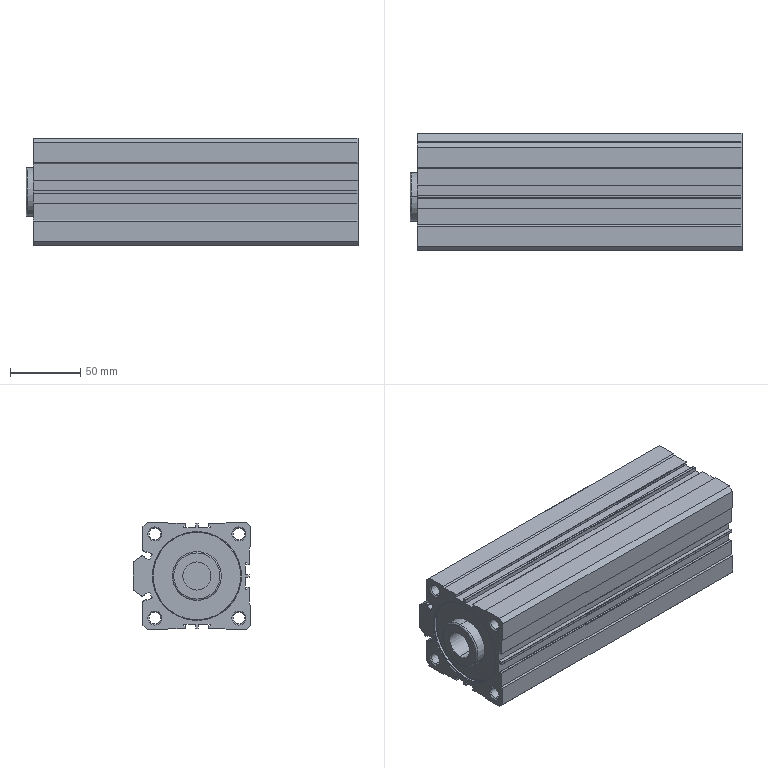Part | SolidWorks | features BaseBody 1 | 1 solid | 202 faces | box 237 x 84 x 77 mm | volume 632926 mm3 | plane 84 | cylinder 78 | cone 32 | torus 8 | commonest cylinder face diameters 0.4 x35 0.8 x15 8.376 x8 63 x8 64 x4 20 x2